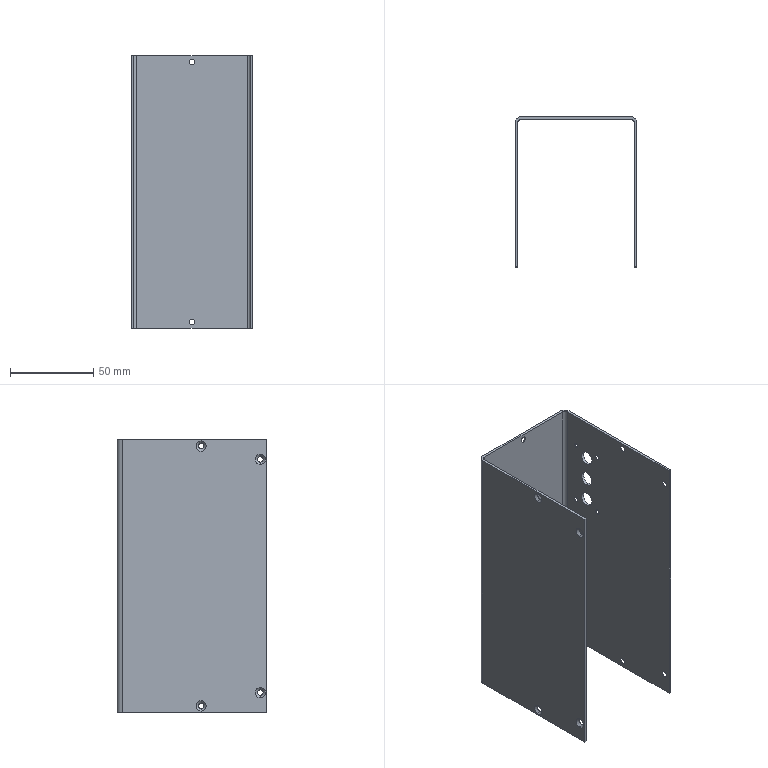Part | SolidWorks | features BaseBody 1 | 1 solid | 160 faces | box 73.2 x 90 x 163.5 mm | volume 60174 mm3 | plane 82 | cylinder 38 | cone 28 | spline 12 | commonest cylinder face diameters 3.4 x20 2.8 x8 8.5 x6 4 x2 7 x2